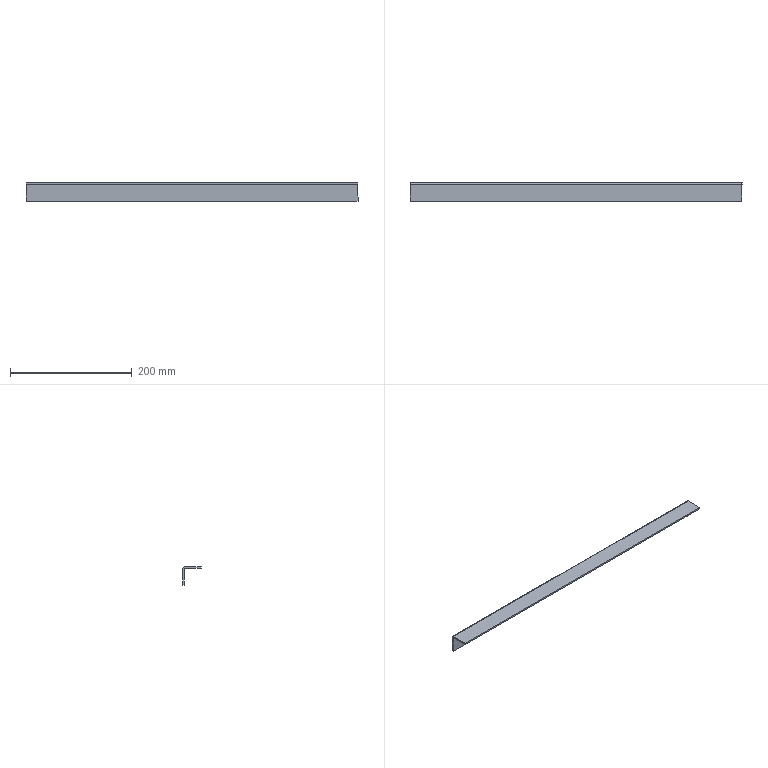Part | SolidWorks | features EdgeFlange 1, FlatPattern 1, SMBaseFlange 1, SheetMetal 1 | 1 solid | 14 faces | box 546 x 30 x 30 mm | volume 77462 mm3 | plane 12 | cylinder 2 | commonest cylinder face diameters 1 x1 6 x1
STEP:
#1=CARTESIAN_POINT('',(273.,-15.,-2.5));
#2=VERTEX_POINT('',#1);
#3=CARTESIAN_POINT('',(273.,12.,-2.5));
#4=VERTEX_POINT('',#3);
#5=CARTESIAN_POINT('',(273.,15.,-2.5));
#6=DIRECTION('',(0.,1.,0.));
#7=VECTOR('',#6,1000.);
#8=LINE('',#5,#7);
#9=EDGE_CURVE('',#2,#4,#8,.T.);
#10=ORIENTED_EDGE('',*,*,#9,.T.);
#11=CARTESIAN_POINT('',(273.,12.,0.));
#12=VERTEX_POINT('',#11);
#13=CARTESIAN_POINT('',(273.,12.,-2.5));
#14=DIRECTION('',(0.,0.,1.));
#15=VECTOR('',#14,1000.);
#16=LINE('',#13,#15);
#17=EDGE_CURVE('',#4,#12,#16,.T.);
#18=ORIENTED_EDGE('',*,*,#17,.T.);
#19=CARTESIAN_POINT('',(273.,-15.,0.));
#20=VERTEX_POINT('',#19);
#21=CARTESIAN_POINT('',(273.,15.,0.));
#22=DIRECTION('',(0.,1.,0.));
#23=VECTOR('',#22,1000.);
#24=LINE('',#21,#23);
#25=EDGE_CURVE('',#20,#12,#24,.T.);
#26=ORIENTED_EDGE('',*,*,#25,.F.);
#27=CARTESIAN_POINT('',(273.,-15.,-2.5));
#28=DIRECTION('',(0.,0.,1.));
#29=VECTOR('',#28,1000.);
#30=LINE('',#27,#29);
#31=EDGE_CURVE('',#2,#20,#30,.T.);
#32=ORIENTED_EDGE('',*,*,#31,.F.);
#33=EDGE_LOOP('',(#10,#18,#26,#32));
#34=FACE_OUTER_BOUND('',#33,.T.);
#35=CARTESIAN_POINT('',(273.,15.,-2.5));
#36=DIRECTION('',(1.,0.,0.));
#37=DIRECTION('',(0.,0.,-1.));
#38=AXIS2_PLACEMENT_3D('',#35,#36,#37);
#39=PLANE('',#38);
#40=ADVANCED_FACE('',(#34),#39,.T.);
#41=CARTESIAN_POINT('',(-273.,12.,-2.5));
#42=VERTEX_POINT('',#41);
#43=CARTESIAN_POINT('',(273.,12.,-2.5));
#44=DIRECTION('',(-1.,0.,0.));
#45=VECTOR('',#44,1000.);
#46=LINE('',#43,#45);
#47=EDGE_CURVE('',#4,#42,#46,.T.);
#48=ORIENTED_EDGE('',*,*,#47,.F.);
#49=ORIENTED_EDGE('',*,*,#9,.F.);
#50=CARTESIAN_POINT('',(-273.,-15.,-2.5));
#51=VERTEX_POINT('',#50);
#52=CARTESIAN_POINT('',(-273.,-15.,-2.5));
#53=DIRECTION('',(1.,0.,0.));
#54=VECTOR('',#53,1000.);
#55=LINE('',#52,#54);
#56=EDGE_CURVE('',#51,#2,#55,.T.);
#57=ORIENTED_EDGE('',*,*,#56,.F.);
#58=CARTESIAN_POINT('',(-273.,15.,-2.5));
#59=DIRECTION('',(0.,-1.,0.));
#60=VECTOR('',#59,1000.);
#61=LINE('',#58,#60);
#62=EDGE_CURVE('',#42,#51,#61,.T.);
#63=ORIENTED_EDGE('',*,*,#62,.F.);
#64=EDGE_LOOP('',(#48,#49,#57,#63));
#65=FACE_OUTER_BOUND('',#64,.T.);
#66=CARTESIAN_POINT('',(0.,0.,-2.5));
#67=DIRECTION('',(0.,0.,1.));
#68=DIRECTION('',(1.,0.,0.));
#69=AXIS2_PLACEMENT_3D('',#66,#67,#68);
#70=PLANE('',#69);
#71=ADVANCED_FACE('',(#65),#70,.F.);
#72=ORIENTED_EDGE('',*,*,#25,.T.);
#73=CARTESIAN_POINT('',(-273.,12.,0.));
#74=VERTEX_POINT('',#73);
#75=CARTESIAN_POINT('',(273.,12.,0.));
#76=DIRECTION('',(-1.,0.,0.));
#77=VECTOR('',#76,1000.);
#78=LINE('',#75,#77);
#79=EDGE_CURVE('',#12,#74,#78,.T.);
#80=ORIENTED_EDGE('',*,*,#79,.T.);
#81=CARTESIAN_POINT('',(-273.,-15.,0.));
#82=VERTEX_POINT('',#81);
#83=CARTESIAN_POINT('',(-273.,15.,0.));
#84=DIRECTION('',(0.,-1.,0.));
#85=VECTOR('',#84,1000.);
#86=LINE('',#83,#85);
#87=EDGE_CURVE('',#74,#82,#86,.T.);
#88=ORIENTED_EDGE('',*,*,#87,.T.);
#89=CARTESIAN_POINT('',(-273.,-15.,0.));
#90=DIRECTION('',(1.,0.,0.));
#91=VECTOR('',#90,1000.);
#92=LINE('',#89,#91);
#93=EDGE_CURVE('',#82,#20,#92,.T.);
#94=ORIENTED_EDGE('',*,*,#93,.T.);
#95=EDGE_LOOP('',(#72,#80,#88,#94));
#96=FACE_OUTER_BOUND('',#95,.T.);
#97=CARTESIAN_POINT('',(0.,0.,0.));
#98=DIRECTION('',(0.,0.,1.));
#99=DIRECTION('',(1.,0.,0.));
#100=AXIS2_PLACEMENT_3D('',#97,#98,#99);
#101=PLANE('',#100);
#102=ADVANCED_FACE('',(#96),#101,.T.);
#103=ORIENTED_EDGE('',*,*,#93,.F.);
#104=CARTESIAN_POINT('',(-273.,-15.,-2.5));
#105=DIRECTION('',(0.,0.,1.));
#106=VECTOR('',#105,1000.);
#107=LINE('',#104,#106);
#108=EDGE_CURVE('',#51,#82,#107,.T.);
#109=ORIENTED_EDGE('',*,*,#108,.F.);
#110=ORIENTED_EDGE('',*,*,#56,.T.);
#111=ORIENTED_EDGE('',*,*,#31,.T.);
#112=EDGE_LOOP('',(#103,#109,#110,#111));
#113=FACE_OUTER_BOUND('',#112,.T.);
#114=CARTESIAN_POINT('',(-273.,-15.,-2.5));
#115=DIRECTION('',(0.,-1.,0.));
#116=DIRECTION('',(0.,0.,-1.));
#117=AXIS2_PLACEMENT_3D('',#114,#115,#116);
#118=PLANE('',#117);
#119=ADVANCED_FACE('',(#113),#118,.T.);
#120=CARTESIAN_POINT('',(-273.,12.,-2.5));
#121=DIRECTION('',(0.,0.,1.));
#122=VECTOR('',#121,1000.);
#123=LINE('',#120,#122);
#124=EDGE_CURVE('',#42,#74,#123,.T.);
#125=ORIENTED_EDGE('',*,*,#124,.F.);
#126=ORIENTED_EDGE('',*,*,#62,.T.);
#127=ORIENTED_EDGE('',*,*,#108,.T.);
#128=ORIENTED_EDGE('',*,*,#87,.F.);
#129=EDGE_LOOP('',(#125,#126,#127,#128));
#130=FACE_OUTER_BOUND('',#129,.T.);
#131=CARTESIAN_POINT('',(-273.,15.,-2.5));
#132=DIRECTION('',(-1.,0.,0.));
#133=DIRECTION('',(0.,0.,1.));
#134=AXIS2_PLACEMENT_3D('',#131,#132,#133);
#135=PLANE('',#134);
#136=ADVANCED_FACE('',(#130),#135,.T.);
#137=CARTESIAN_POINT('',(-273.,12.5,-3.));
#138=VERTEX_POINT('',#137);
#139=CARTESIAN_POINT('',(-273.,15.,-3.));
#140=VERTEX_POINT('',#139);
#141=CARTESIAN_POINT('',(-273.,15.,-3.));
#142=DIRECTION('',(0.,1.,0.));
#143=VECTOR('',#142,1000.);
#144=LINE('',#141,#143);
#145=EDGE_CURVE('',#138,#140,#144,.T.);
#146=ORIENTED_EDGE('',*,*,#145,.F.);
#147=CARTESIAN_POINT('',(-273.,12.,-3.));
#148=DIRECTION('',(-1.,0.,0.));
#149=DIRECTION('',(0.,0.,-1.));
#150=AXIS2_PLACEMENT_3D('',#147,#148,#149);
#151=CIRCLE('',#150,0.5);
#152=EDGE_CURVE('',#42,#138,#151,.T.);
#153=ORIENTED_EDGE('',*,*,#152,.F.);
#154=ORIENTED_EDGE('',*,*,#124,.T.);
#155=CARTESIAN_POINT('',(-273.,12.,-3.));
#156=DIRECTION('',(-1.,0.,0.));
#157=DIRECTION('',(0.,0.,-1.));
#158=AXIS2_PLACEMENT_3D('',#155,#156,#157);
#159=CIRCLE('',#158,3.);
#160=EDGE_CURVE('',#74,#140,#159,.T.);
#161=ORIENTED_EDGE('',*,*,#160,.T.);
#162=EDGE_LOOP('',(#146,#153,#154,#161));
#163=FACE_OUTER_BOUND('',#162,.T.);
#164=CARTESIAN_POINT('',(-273.,12.,-3.));
#165=DIRECTION('',(-1.,0.,0.));
#166=DIRECTION('',(0.,0.,1.));
#167=AXIS2_PLACEMENT_3D('',#164,#165,#166);
#168=PLANE('',#167);
#169=ADVANCED_FACE('',(#163),#168,.T.);
#170=CARTESIAN_POINT('',(273.,12.5,-3.));
#171=VERTEX_POINT('',#170);
#172=CARTESIAN_POINT('',(273.,12.,-3.));
#173=DIRECTION('',(1.,0.,0.));
#174=DIRECTION('',(0.,0.,-1.));
#175=AXIS2_PLACEMENT_3D('',#172,#173,#174);
#176=CIRCLE('',#175,0.5);
#177=EDGE_CURVE('',#171,#4,#176,.T.);
#178=ORIENTED_EDGE('',*,*,#177,.F.);
#179=CARTESIAN_POINT('',(273.,15.,-3.));
#180=VERTEX_POINT('',#179);
#181=CARTESIAN_POINT('',(273.,12.5,-3.));
#182=DIRECTION('',(0.,1.,0.));
#183=VECTOR('',#182,1000.);
#184=LINE('',#181,#183);
#185=EDGE_CURVE('',#171,#180,#184,.T.);
#186=ORIENTED_EDGE('',*,*,#185,.T.);
#187=CARTESIAN_POINT('',(273.,12.,-3.));
#188=DIRECTION('',(1.,0.,0.));
#189=DIRECTION('',(0.,0.,-1.));
#190=AXIS2_PLACEMENT_3D('',#187,#188,#189);
#191=CIRCLE('',#190,3.);
#192=EDGE_CURVE('',#180,#12,#191,.T.);
#193=ORIENTED_EDGE('',*,*,#192,.T.);
#194=ORIENTED_EDGE('',*,*,#17,.F.);
#195=EDGE_LOOP('',(#178,#186,#193,#194));
#196=FACE_OUTER_BOUND('',#195,.T.);
#197=CARTESIAN_POINT('',(273.,12.,-3.));
#198=DIRECTION('',(-1.,0.,0.));
#199=DIRECTION('',(0.,0.,1.));
#200=AXIS2_PLACEMENT_3D('',#197,#198,#199);
#201=PLANE('',#200);
#202=ADVANCED_FACE('',(#196),#201,.F.);
#203=ORIENTED_EDGE('',*,*,#79,.F.);
#204=ORIENTED_EDGE('',*,*,#192,.F.);
#205=CARTESIAN_POINT('',(0.,15.,-3.));
#206=DIRECTION('',(1.,0.,0.));
#207=VECTOR('',#206,1000.);
#208=LINE('',#205,#207);
#209=EDGE_CURVE('',#140,#180,#208,.T.);
#210=ORIENTED_EDGE('',*,*,#209,.F.);
#211=ORIENTED_EDGE('',*,*,#160,.F.);
#212=EDGE_LOOP('',(#203,#204,#210,#211));
#213=FACE_OUTER_BOUND('',#212,.T.);
#214=CARTESIAN_POINT('',(273.,12.,-3.));
#215=DIRECTION('',(1.,0.,0.));
#216=DIRECTION('',(0.,1.,0.));
#217=AXIS2_PLACEMENT_3D('',#214,#215,#216);
#218=CYLINDRICAL_SURFACE('',#217,3.);
#219=ADVANCED_FACE('',(#213),#218,.T.);
#220=ORIENTED_EDGE('',*,*,#47,.T.);
#221=ORIENTED_EDGE('',*,*,#152,.T.);
#222=CARTESIAN_POINT('',(-273.,12.5,-3.));
#223=DIRECTION('',(1.,0.,0.));
#224=VECTOR('',#223,1000.);
#225=LINE('',#222,#224);
#226=EDGE_CURVE('',#138,#171,#225,.T.);
#227=ORIENTED_EDGE('',*,*,#226,.T.);
#228=ORIENTED_EDGE('',*,*,#177,.T.);
#229=EDGE_LOOP('',(#220,#221,#227,#228));
#230=FACE_OUTER_BOUND('',#229,.T.);
#231=CARTESIAN_POINT('',(273.,12.,-3.));
#232=DIRECTION('',(1.,0.,0.));
#233=DIRECTION('',(0.,1.,0.));
#234=AXIS2_PLACEMENT_3D('',#231,#232,#233);
#235=CYLINDRICAL_SURFACE('',#234,0.5);
#236=ADVANCED_FACE('',(#230),#235,.F.);
#237=CARTESIAN_POINT('',(273.,15.,-30.));
#238=VERTEX_POINT('',#237);
#239=CARTESIAN_POINT('',(273.,15.,-2.5));
#240=DIRECTION('',(0.,0.,1.));
#241=VECTOR('',#240,1000.);
#242=LINE('',#239,#241);
#243=EDGE_CURVE('',#238,#180,#242,.T.);
#244=ORIENTED_EDGE('',*,*,#243,.T.);
#245=ORIENTED_EDGE('',*,*,#185,.F.);
#246=CARTESIAN_POINT('',(273.,12.5,-30.));
#247=VERTEX_POINT('',#246);
#248=CARTESIAN_POINT('',(273.,12.5,0.));
#249=DIRECTION('',(0.,0.,1.));
#250=VECTOR('',#249,1000.);
#251=LINE('',#248,#250);
#252=EDGE_CURVE('',#247,#171,#251,.T.);
#253=ORIENTED_EDGE('',*,*,#252,.F.);
#254=CARTESIAN_POINT('',(273.,15.,-30.));
#255=DIRECTION('',(0.,-1.,0.));
#256=VECTOR('',#255,1000.);
#257=LINE('',#254,#256);
#258=EDGE_CURVE('',#238,#247,#257,.T.);
#259=ORIENTED_EDGE('',*,*,#258,.F.);
#260=EDGE_LOOP('',(#244,#245,#253,#259));
#261=FACE_OUTER_BOUND('',#260,.T.);
#262=CARTESIAN_POINT('',(273.,15.,-2.5));
#263=DIRECTION('',(1.,0.,0.));
#264=DIRECTION('',(0.,0.,-1.));
#265=AXIS2_PLACEMENT_3D('',#262,#263,#264);
#266=PLANE('',#265);
#267=ADVANCED_FACE('',(#261),#266,.T.);
#268=CARTESIAN_POINT('',(-273.,12.5,-30.));
#269=VERTEX_POINT('',#268);
#270=CARTESIAN_POINT('',(-273.,12.5,0.));
#271=DIRECTION('',(0.,0.,-1.));
#272=VECTOR('',#271,1000.);
#273=LINE('',#270,#272);
#274=EDGE_CURVE('',#138,#269,#273,.T.);
#275=ORIENTED_EDGE('',*,*,#274,.F.);
#276=ORIENTED_EDGE('',*,*,#145,.T.);
#277=CARTESIAN_POINT('',(-273.,15.,-30.));
#278=VERTEX_POINT('',#277);
#279=CARTESIAN_POINT('',(-273.,15.,-30.));
#280=DIRECTION('',(0.,0.,-1.));
#281=VECTOR('',#280,1000.);
#282=LINE('',#279,#281);
#283=EDGE_CURVE('',#140,#278,#282,.T.);
#284=ORIENTED_EDGE('',*,*,#283,.T.);
#285=CARTESIAN_POINT('',(-273.,15.,-30.));
#286=DIRECTION('',(0.,-1.,0.));
#287=VECTOR('',#286,1000.);
#288=LINE('',#285,#287);
#289=EDGE_CURVE('',#278,#269,#288,.T.);
#290=ORIENTED_EDGE('',*,*,#289,.T.);
#291=EDGE_LOOP('',(#275,#276,#284,#290));
#292=FACE_OUTER_BOUND('',#291,.T.);
#293=CARTESIAN_POINT('',(-273.,15.,-30.));
#294=DIRECTION('',(-1.,0.,0.));
#295=DIRECTION('',(0.,0.,1.));
#296=AXIS2_PLACEMENT_3D('',#293,#294,#295);
#297=PLANE('',#296);
#298=ADVANCED_FACE('',(#292),#297,.T.);
#299=ORIENTED_EDGE('',*,*,#283,.F.);
#300=ORIENTED_EDGE('',*,*,#209,.T.);
#301=ORIENTED_EDGE('',*,*,#243,.F.);
#302=CARTESIAN_POINT('',(273.,15.,-30.));
#303=DIRECTION('',(1.,0.,0.));
#304=VECTOR('',#303,1000.);
#305=LINE('',#302,#304);
#306=EDGE_CURVE('',#278,#238,#305,.T.);
#307=ORIENTED_EDGE('',*,*,#306,.F.);
#308=EDGE_LOOP('',(#299,#300,#301,#307));
#309=FACE_OUTER_BOUND('',#308,.T.);
#310=CARTESIAN_POINT('',(0.,15.,0.));
#311=DIRECTION('',(0.,1.,0.));
#312=DIRECTION('',(0.,0.,1.));
#313=AXIS2_PLACEMENT_3D('',#310,#311,#312);
#314=PLANE('',#313);
#315=ADVANCED_FACE('',(#309),#314,.T.);
#316=ORIENTED_EDGE('',*,*,#226,.F.);
#317=ORIENTED_EDGE('',*,*,#274,.T.);
#318=CARTESIAN_POINT('',(0.,12.5,-30.));
#319=DIRECTION('',(1.,0.,0.));
#320=VECTOR('',#319,1000.);
#321=LINE('',#318,#320);
#322=EDGE_CURVE('',#269,#247,#321,.T.);
#323=ORIENTED_EDGE('',*,*,#322,.T.);
#324=ORIENTED_EDGE('',*,*,#252,.T.);
#325=EDGE_LOOP('',(#316,#317,#323,#324));
#326=FACE_OUTER_BOUND('',#325,.T.);
#327=CARTESIAN_POINT('',(0.,12.5,0.));
#328=DIRECTION('',(0.,1.,0.));
#329=DIRECTION('',(0.,0.,1.));
#330=AXIS2_PLACEMENT_3D('',#327,#328,#329);
#331=PLANE('',#330);
#332=ADVANCED_FACE('',(#326),#331,.F.);
#333=ORIENTED_EDGE('',*,*,#322,.F.);
#334=ORIENTED_EDGE('',*,*,#289,.F.);
#335=ORIENTED_EDGE('',*,*,#306,.T.);
#336=ORIENTED_EDGE('',*,*,#258,.T.);
#337=EDGE_LOOP('',(#333,#334,#335,#336));
#338=FACE_OUTER_BOUND('',#337,.T.);
#339=CARTESIAN_POINT('',(273.,15.,-30.));
#340=DIRECTION('',(0.,0.,-1.));
#341=DIRECTION('',(0.,1.,0.));
#342=AXIS2_PLACEMENT_3D('',#339,#340,#341);
#343=PLANE('',#342);
#344=ADVANCED_FACE('',(#338),#343,.T.);
#345=CLOSED_SHELL('',(#40,#71,#102,#119,#136,#169,#202,#219,#236,#267,#298,#315,#332,#344));
#346=MANIFOLD_SOLID_BREP('',#345);
#347=CARTESIAN_POINT('',(0.,0.,0.));
#348=DIRECTION('',(0.,0.,1.));
#349=DIRECTION('',(1.,0.,0.));
#350=AXIS2_PLACEMENT_3D('',#347,#348,#349);
#351=(LENGTH_UNIT()NAMED_UNIT(*)SI_UNIT(.MILLI.,.METRE.));
#352=UNCERTAINTY_MEASURE_WITH_UNIT(LENGTH_MEASURE(0.00001),#351,'','');
#353=(NAMED_UNIT(*)PLANE_ANGLE_UNIT()SI_UNIT($,.RADIAN.));
#354=(NAMED_UNIT(*)SI_UNIT($,.STERADIAN.)SOLID_ANGLE_UNIT());
#355=(GEOMETRIC_REPRESENTATION_CONTEXT(3)GLOBAL_UNCERTAINTY_ASSIGNED_CONTEXT((#352))GLOBAL_UNIT_ASSIGNED_CONTEXT((#351,#353,#354))REPRESENTATION_CONTEXT('',''));
#356=ADVANCED_BREP_SHAPE_REPRESENTATION('',(#346,#350),#355);